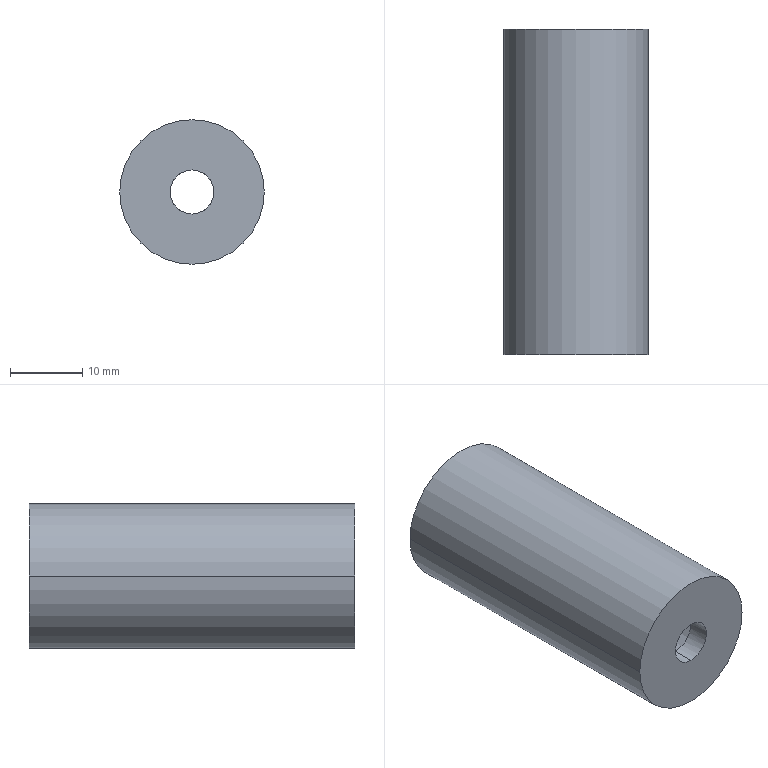Part | NX | features BREP 1 | 1 solid | 12 faces | box 19.99 x 44.958 x 19.99 mm | volume 9059 mm3 | cylinder 6 | cone 4 | plane 2 | commonest cylinder face diameters 6.096 x2 12.294 x2 19.99 x2
STEP:
#1=CARTESIAN_POINT('',(-9.995,0.,0.));
#2=VERTEX_POINT('',#1);
#3=CARTESIAN_POINT('',(9.995,0.,0.));
#4=VERTEX_POINT('',#3);
#5=CARTESIAN_POINT('',(0.,0.,0.));
#6=DIRECTION('',(0.,1.,0.));
#7=DIRECTION('',(-1.,0.,0.));
#8=AXIS2_PLACEMENT_3D('',#5,#6,#7);
#9=CIRCLE('',#8,9.995);
#10=EDGE_CURVE('',#2,#4,#9,.T.);
#11=ORIENTED_EDGE('',*,*,#10,.F.);
#12=CARTESIAN_POINT('',(0.,0.,0.));
#13=DIRECTION('',(0.,1.,0.));
#14=DIRECTION('',(1.,0.,0.));
#15=AXIS2_PLACEMENT_3D('',#12,#13,#14);
#16=CIRCLE('',#15,9.995);
#17=EDGE_CURVE('',#4,#2,#16,.T.);
#18=ORIENTED_EDGE('',*,*,#17,.F.);
#19=EDGE_LOOP('',(#11,#18));
#20=FACE_BOUND('',#19,.T.);
#21=CARTESIAN_POINT('',(0.,0.,3.048));
#22=VERTEX_POINT('',#21);
#23=CARTESIAN_POINT('',(0.,0.,-3.048));
#24=VERTEX_POINT('',#23);
#25=CARTESIAN_POINT('',(0.,0.,0.));
#26=DIRECTION('',(0.,-1.,0.));
#27=DIRECTION('',(0.,0.,1.));
#28=AXIS2_PLACEMENT_3D('',#25,#26,#27);
#29=CIRCLE('',#28,3.048);
#30=EDGE_CURVE('',#22,#24,#29,.T.);
#31=ORIENTED_EDGE('',*,*,#30,.F.);
#32=CARTESIAN_POINT('',(0.,0.,0.));
#33=DIRECTION('',(0.,-1.,0.));
#34=DIRECTION('',(0.,0.,-1.));
#35=AXIS2_PLACEMENT_3D('',#32,#33,#34);
#36=CIRCLE('',#35,3.048);
#37=EDGE_CURVE('',#24,#22,#36,.T.);
#38=ORIENTED_EDGE('',*,*,#37,.F.);
#39=EDGE_LOOP('',(#31,#38));
#40=FACE_BOUND('',#39,.T.);
#41=CARTESIAN_POINT('',(0.,0.,0.));
#42=DIRECTION('',(0.,1.,0.));
#43=DIRECTION('',(1.,0.,0.));
#44=AXIS2_PLACEMENT_3D('',#41,#42,#43);
#45=PLANE('',#44);
#46=ADVANCED_FACE('',(#20,#40),#45,.F.);
#47=CARTESIAN_POINT('',(-9.995,44.958,0.));
#48=VERTEX_POINT('',#47);
#49=CARTESIAN_POINT('',(-9.995,0.,0.));
#50=DIRECTION('',(0.,1.,0.));
#51=VECTOR('',#50,1000.);
#52=LINE('',#49,#51);
#53=EDGE_CURVE('',#2,#48,#52,.T.);
#54=ORIENTED_EDGE('',*,*,#53,.T.);
#55=CARTESIAN_POINT('',(9.995,44.958,0.));
#56=VERTEX_POINT('',#55);
#57=CARTESIAN_POINT('',(0.,44.958,0.));
#58=DIRECTION('',(0.,1.,0.));
#59=DIRECTION('',(1.,0.,0.));
#60=AXIS2_PLACEMENT_3D('',#57,#58,#59);
#61=CIRCLE('',#60,9.995);
#62=EDGE_CURVE('',#56,#48,#61,.T.);
#63=ORIENTED_EDGE('',*,*,#62,.F.);
#64=CARTESIAN_POINT('',(9.995,0.,0.));
#65=DIRECTION('',(0.,1.,0.));
#66=VECTOR('',#65,1000.);
#67=LINE('',#64,#66);
#68=EDGE_CURVE('',#4,#56,#67,.T.);
#69=ORIENTED_EDGE('',*,*,#68,.F.);
#70=ORIENTED_EDGE('',*,*,#17,.T.);
#71=EDGE_LOOP('',(#54,#63,#69,#70));
#72=FACE_BOUND('',#71,.T.);
#73=CARTESIAN_POINT('',(0.,0.,0.));
#74=DIRECTION('',(0.,1.,0.));
#75=DIRECTION('',(1.,0.,0.));
#76=AXIS2_PLACEMENT_3D('',#73,#74,#75);
#77=CYLINDRICAL_SURFACE('',#76,9.995);
#78=ADVANCED_FACE('',(#72),#77,.T.);
#79=ORIENTED_EDGE('',*,*,#68,.T.);
#80=CARTESIAN_POINT('',(0.,44.958,0.));
#81=DIRECTION('',(0.,1.,0.));
#82=DIRECTION('',(-1.,0.,0.));
#83=AXIS2_PLACEMENT_3D('',#80,#81,#82);
#84=CIRCLE('',#83,9.995);
#85=EDGE_CURVE('',#48,#56,#84,.T.);
#86=ORIENTED_EDGE('',*,*,#85,.F.);
#87=ORIENTED_EDGE('',*,*,#53,.F.);
#88=ORIENTED_EDGE('',*,*,#10,.T.);
#89=EDGE_LOOP('',(#79,#86,#87,#88));
#90=FACE_BOUND('',#89,.T.);
#91=CARTESIAN_POINT('',(0.,0.,0.));
#92=DIRECTION('',(0.,1.,0.));
#93=DIRECTION('',(1.,0.,0.));
#94=AXIS2_PLACEMENT_3D('',#91,#92,#93);
#95=CYLINDRICAL_SURFACE('',#94,9.995);
#96=ADVANCED_FACE('',(#90),#95,.T.);
#97=ORIENTED_EDGE('',*,*,#85,.T.);
#98=ORIENTED_EDGE('',*,*,#62,.T.);
#99=EDGE_LOOP('',(#97,#98));
#100=FACE_BOUND('',#99,.T.);
#101=CARTESIAN_POINT('',(-8.179,44.958,0.));
#102=VERTEX_POINT('',#101);
#103=CARTESIAN_POINT('',(8.179,44.958,0.));
#104=VERTEX_POINT('',#103);
#105=CARTESIAN_POINT('',(0.,44.958,0.));
#106=DIRECTION('',(0.,1.,0.));
#107=DIRECTION('',(-1.,0.,0.));
#108=AXIS2_PLACEMENT_3D('',#105,#106,#107);
#109=CIRCLE('',#108,8.179);
#110=EDGE_CURVE('',#102,#104,#109,.T.);
#111=ORIENTED_EDGE('',*,*,#110,.F.);
#112=CARTESIAN_POINT('',(0.,44.958,0.));
#113=DIRECTION('',(0.,1.,0.));
#114=DIRECTION('',(1.,0.,0.));
#115=AXIS2_PLACEMENT_3D('',#112,#113,#114);
#116=CIRCLE('',#115,8.179);
#117=EDGE_CURVE('',#104,#102,#116,.T.);
#118=ORIENTED_EDGE('',*,*,#117,.F.);
#119=EDGE_LOOP('',(#111,#118));
#120=FACE_BOUND('',#119,.T.);
#121=CARTESIAN_POINT('',(0.,44.958,0.));
#122=DIRECTION('',(0.,1.,0.));
#123=DIRECTION('',(1.,0.,0.));
#124=AXIS2_PLACEMENT_3D('',#121,#122,#123);
#125=PLANE('',#124);
#126=ADVANCED_FACE('',(#100,#120),#125,.T.);
#127=CARTESIAN_POINT('',(-6.147,42.926,0.));
#128=VERTEX_POINT('',#127);
#129=CARTESIAN_POINT('',(-8.179,44.958,0.));
#130=DIRECTION('',(0.7071,-0.7071,0.));
#131=VECTOR('',#130,1000.);
#132=LINE('',#129,#131);
#133=EDGE_CURVE('',#102,#128,#132,.T.);
#134=ORIENTED_EDGE('',*,*,#133,.T.);
#135=CARTESIAN_POINT('',(6.147,42.926,0.));
#136=VERTEX_POINT('',#135);
#137=CARTESIAN_POINT('',(0.,42.926,0.));
#138=DIRECTION('',(0.,1.,0.));
#139=DIRECTION('',(1.,0.,0.));
#140=AXIS2_PLACEMENT_3D('',#137,#138,#139);
#141=CIRCLE('',#140,6.147);
#142=EDGE_CURVE('',#136,#128,#141,.T.);
#143=ORIENTED_EDGE('',*,*,#142,.F.);
#144=CARTESIAN_POINT('',(8.179,44.958,0.));
#145=DIRECTION('',(-0.7071,-0.7071,0.));
#146=VECTOR('',#145,1000.);
#147=LINE('',#144,#146);
#148=EDGE_CURVE('',#104,#136,#147,.T.);
#149=ORIENTED_EDGE('',*,*,#148,.F.);
#150=ORIENTED_EDGE('',*,*,#117,.T.);
#151=EDGE_LOOP('',(#134,#143,#149,#150));
#152=FACE_BOUND('',#151,.T.);
#153=CARTESIAN_POINT('',(0.,43.942,0.));
#154=DIRECTION('',(0.,1.,0.));
#155=DIRECTION('',(1.,0.,0.));
#156=AXIS2_PLACEMENT_3D('',#153,#154,#155);
#157=CONICAL_SURFACE('',#156,7.163,0.7854);
#158=ADVANCED_FACE('',(#152),#157,.F.);
#159=ORIENTED_EDGE('',*,*,#148,.T.);
#160=CARTESIAN_POINT('',(0.,42.926,0.));
#161=DIRECTION('',(0.,1.,0.));
#162=DIRECTION('',(-1.,0.,0.));
#163=AXIS2_PLACEMENT_3D('',#160,#161,#162);
#164=CIRCLE('',#163,6.147);
#165=EDGE_CURVE('',#128,#136,#164,.T.);
#166=ORIENTED_EDGE('',*,*,#165,.F.);
#167=ORIENTED_EDGE('',*,*,#133,.F.);
#168=ORIENTED_EDGE('',*,*,#110,.T.);
#169=EDGE_LOOP('',(#159,#166,#167,#168));
#170=FACE_BOUND('',#169,.T.);
#171=CARTESIAN_POINT('',(0.,43.942,0.));
#172=DIRECTION('',(0.,1.,0.));
#173=DIRECTION('',(1.,0.,0.));
#174=AXIS2_PLACEMENT_3D('',#171,#172,#173);
#175=CONICAL_SURFACE('',#174,7.163,0.7854);
#176=ADVANCED_FACE('',(#170),#175,.F.);
#177=CARTESIAN_POINT('',(-6.147,5.08,0.));
#178=VERTEX_POINT('',#177);
#179=CARTESIAN_POINT('',(-6.147,42.926,0.));
#180=DIRECTION('',(0.,-1.,0.));
#181=VECTOR('',#180,1000.);
#182=LINE('',#179,#181);
#183=EDGE_CURVE('',#128,#178,#182,.T.);
#184=ORIENTED_EDGE('',*,*,#183,.F.);
#185=ORIENTED_EDGE('',*,*,#165,.T.);
#186=CARTESIAN_POINT('',(6.147,5.08,0.));
#187=VERTEX_POINT('',#186);
#188=CARTESIAN_POINT('',(6.147,42.926,0.));
#189=DIRECTION('',(0.,-1.,0.));
#190=VECTOR('',#189,1000.);
#191=LINE('',#188,#190);
#192=EDGE_CURVE('',#136,#187,#191,.T.);
#193=ORIENTED_EDGE('',*,*,#192,.T.);
#194=CARTESIAN_POINT('',(0.,5.08,0.));
#195=DIRECTION('',(0.,1.,0.));
#196=DIRECTION('',(-1.,0.,0.));
#197=AXIS2_PLACEMENT_3D('',#194,#195,#196);
#198=CIRCLE('',#197,6.147);
#199=EDGE_CURVE('',#178,#187,#198,.T.);
#200=ORIENTED_EDGE('',*,*,#199,.F.);
#201=EDGE_LOOP('',(#184,#185,#193,#200));
#202=FACE_BOUND('',#201,.T.);
#203=CARTESIAN_POINT('',(0.,44.958,0.));
#204=DIRECTION('',(0.,1.,0.));
#205=DIRECTION('',(1.,0.,0.));
#206=AXIS2_PLACEMENT_3D('',#203,#204,#205);
#207=CYLINDRICAL_SURFACE('',#206,6.147);
#208=ADVANCED_FACE('',(#202),#207,.F.);
#209=CARTESIAN_POINT('',(3.048,3.048,0.));
#210=VERTEX_POINT('',#209);
#211=CARTESIAN_POINT('',(3.048,3.048,0.));
#212=DIRECTION('',(0.8362,0.5484,0.));
#213=VECTOR('',#212,1000.);
#214=LINE('',#211,#213);
#215=EDGE_CURVE('',#187,#210,#214,.F.);
#216=ORIENTED_EDGE('',*,*,#215,.T.);
#217=CARTESIAN_POINT('',(0.,3.048,3.048));
#218=VERTEX_POINT('',#217);
#219=CARTESIAN_POINT('',(0.,3.048,0.));
#220=DIRECTION('',(0.,-1.,0.));
#221=DIRECTION('',(1.,0.,0.));
#222=AXIS2_PLACEMENT_3D('',#219,#220,#221);
#223=CIRCLE('',#222,3.048);
#224=EDGE_CURVE('',#210,#218,#223,.T.);
#225=ORIENTED_EDGE('',*,*,#224,.T.);
#226=CARTESIAN_POINT('',(-3.048,3.048,0.));
#227=VERTEX_POINT('',#226);
#228=CARTESIAN_POINT('',(0.,3.048,0.));
#229=DIRECTION('',(0.,-1.,0.));
#230=DIRECTION('',(0.,0.,1.));
#231=AXIS2_PLACEMENT_3D('',#228,#229,#230);
#232=CIRCLE('',#231,3.048);
#233=EDGE_CURVE('',#218,#227,#232,.T.);
#234=ORIENTED_EDGE('',*,*,#233,.T.);
#235=CARTESIAN_POINT('',(-3.048,3.048,0.));
#236=DIRECTION('',(-0.8362,0.5484,0.));
#237=VECTOR('',#236,1000.);
#238=LINE('',#235,#237);
#239=EDGE_CURVE('',#178,#227,#238,.F.);
#240=ORIENTED_EDGE('',*,*,#239,.F.);
#241=ORIENTED_EDGE('',*,*,#199,.T.);
#242=EDGE_LOOP('',(#216,#225,#234,#240,#241));
#243=FACE_BOUND('',#242,.T.);
#244=CARTESIAN_POINT('',(0.,4.064,0.));
#245=DIRECTION('',(0.,1.,0.));
#246=DIRECTION('',(1.,0.,0.));
#247=AXIS2_PLACEMENT_3D('',#244,#245,#246);
#248=CONICAL_SURFACE('',#247,4.597,0.9904);
#249=ADVANCED_FACE('',(#243),#248,.F.);
#250=ORIENTED_EDGE('',*,*,#239,.T.);
#251=CARTESIAN_POINT('',(0.,3.048,-3.048));
#252=VERTEX_POINT('',#251);
#253=CARTESIAN_POINT('',(0.,3.048,0.));
#254=DIRECTION('',(0.,-1.,0.));
#255=DIRECTION('',(-1.,0.,0.));
#256=AXIS2_PLACEMENT_3D('',#253,#254,#255);
#257=CIRCLE('',#256,3.048);
#258=EDGE_CURVE('',#227,#252,#257,.T.);
#259=ORIENTED_EDGE('',*,*,#258,.T.);
#260=CARTESIAN_POINT('',(0.,3.048,0.));
#261=DIRECTION('',(0.,-1.,0.));
#262=DIRECTION('',(0.,0.,-1.));
#263=AXIS2_PLACEMENT_3D('',#260,#261,#262);
#264=CIRCLE('',#263,3.048);
#265=EDGE_CURVE('',#252,#210,#264,.T.);
#266=ORIENTED_EDGE('',*,*,#265,.T.);
#267=ORIENTED_EDGE('',*,*,#215,.F.);
#268=CARTESIAN_POINT('',(0.,5.08,0.));
#269=DIRECTION('',(0.,1.,0.));
#270=DIRECTION('',(1.,0.,0.));
#271=AXIS2_PLACEMENT_3D('',#268,#269,#270);
#272=CIRCLE('',#271,6.147);
#273=EDGE_CURVE('',#187,#178,#272,.T.);
#274=ORIENTED_EDGE('',*,*,#273,.T.);
#275=EDGE_LOOP('',(#250,#259,#266,#267,#274));
#276=FACE_BOUND('',#275,.T.);
#277=CARTESIAN_POINT('',(0.,4.064,0.));
#278=DIRECTION('',(0.,1.,0.));
#279=DIRECTION('',(1.,0.,0.));
#280=AXIS2_PLACEMENT_3D('',#277,#278,#279);
#281=CONICAL_SURFACE('',#280,4.597,0.9904);
#282=ADVANCED_FACE('',(#276),#281,.F.);
#283=ORIENTED_EDGE('',*,*,#192,.F.);
#284=ORIENTED_EDGE('',*,*,#142,.T.);
#285=ORIENTED_EDGE('',*,*,#183,.T.);
#286=ORIENTED_EDGE('',*,*,#273,.F.);
#287=EDGE_LOOP('',(#283,#284,#285,#286));
#288=FACE_BOUND('',#287,.T.);
#289=CARTESIAN_POINT('',(0.,44.958,0.));
#290=DIRECTION('',(0.,1.,0.));
#291=DIRECTION('',(1.,0.,0.));
#292=AXIS2_PLACEMENT_3D('',#289,#290,#291);
#293=CYLINDRICAL_SURFACE('',#292,6.147);
#294=ADVANCED_FACE('',(#288),#293,.F.);
#295=CARTESIAN_POINT('',(0.,0.,-3.048));
#296=DIRECTION('',(0.,1.,0.));
#297=VECTOR('',#296,1000.);
#298=LINE('',#295,#297);
#299=EDGE_CURVE('',#24,#252,#298,.T.);
#300=ORIENTED_EDGE('',*,*,#299,.F.);
#301=ORIENTED_EDGE('',*,*,#37,.T.);
#302=CARTESIAN_POINT('',(0.,0.,3.048));
#303=DIRECTION('',(0.,1.,0.));
#304=VECTOR('',#303,1000.);
#305=LINE('',#302,#304);
#306=EDGE_CURVE('',#22,#218,#305,.T.);
#307=ORIENTED_EDGE('',*,*,#306,.T.);
#308=ORIENTED_EDGE('',*,*,#224,.F.);
#309=ORIENTED_EDGE('',*,*,#265,.F.);
#310=EDGE_LOOP('',(#300,#301,#307,#308,#309));
#311=FACE_BOUND('',#310,.T.);
#312=CARTESIAN_POINT('',(0.,0.,0.));
#313=DIRECTION('',(0.,-1.,0.));
#314=DIRECTION('',(0.,0.,-1.));
#315=AXIS2_PLACEMENT_3D('',#312,#313,#314);
#316=CYLINDRICAL_SURFACE('',#315,3.048);
#317=ADVANCED_FACE('',(#311),#316,.F.);
#318=ORIENTED_EDGE('',*,*,#233,.F.);
#319=ORIENTED_EDGE('',*,*,#306,.F.);
#320=ORIENTED_EDGE('',*,*,#30,.T.);
#321=ORIENTED_EDGE('',*,*,#299,.T.);
#322=ORIENTED_EDGE('',*,*,#258,.F.);
#323=EDGE_LOOP('',(#318,#319,#320,#321,#322));
#324=FACE_BOUND('',#323,.T.);
#325=CARTESIAN_POINT('',(0.,0.,0.));
#326=DIRECTION('',(0.,-1.,0.));
#327=DIRECTION('',(0.,0.,-1.));
#328=AXIS2_PLACEMENT_3D('',#325,#326,#327);
#329=CYLINDRICAL_SURFACE('',#328,3.048);
#330=ADVANCED_FACE('',(#324),#329,.F.);
#331=CLOSED_SHELL('',(#46,#78,#96,#126,#158,#176,#208,#249,#282,#294,#317,#330));
#332=MANIFOLD_SOLID_BREP('',#331);
#333=(LENGTH_UNIT()NAMED_UNIT(*)SI_UNIT(.MILLI.,.METRE.));
#334=UNCERTAINTY_MEASURE_WITH_UNIT(LENGTH_MEASURE(0.00001),#333,'','');
#335=(NAMED_UNIT(*)PLANE_ANGLE_UNIT()SI_UNIT($,.RADIAN.));
#336=(NAMED_UNIT(*)SI_UNIT($,.STERADIAN.)SOLID_ANGLE_UNIT());
#337=(GEOMETRIC_REPRESENTATION_CONTEXT(3)GLOBAL_UNCERTAINTY_ASSIGNED_CONTEXT((#334))GLOBAL_UNIT_ASSIGNED_CONTEXT((#333,#335,#336))REPRESENTATION_CONTEXT('',''));
#338=ADVANCED_BREP_SHAPE_REPRESENTATION('',(#332),#337);